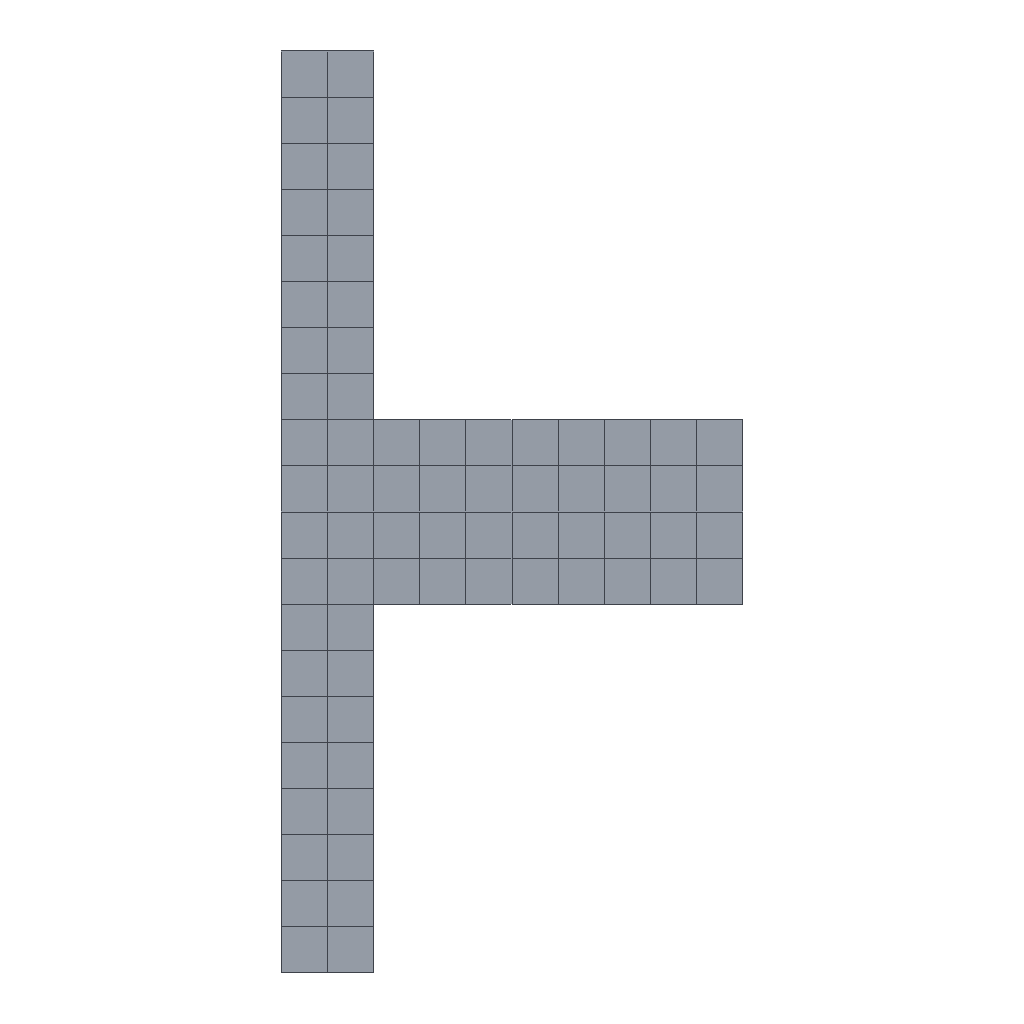Simulation study | abaqus
Set-up summary:
category,name,step,type,value,unit,region
solver,abaqus,,Abaqus/CAE 2024
units,SI m-kg-s (Pa),,inferred,E=2.10439e+11 density=
analysis,deadLoad,,static,nlgeom=True; time_period=1
analysis,heat1,,static,nlgeom=True; time_period=1
analysis,cool1,,static,nlgeom=True; time_period=1
analysis,heat2,,static,nlgeom=True; time_period=1
analysis,cool2,,static,nlgeom=True; time_period=1
analysis,heat3,,static,nlgeom=True; time_period=1
analysis,cool3,,static,nlgeom=True; time_period=1
analysis,heat4,,static,nlgeom=True; time_period=1
analysis,cool4,,static,nlgeom=True; time_period=1
mesh,nodes,,,114
mesh,elements,,,72
element_type,CAX4I,,,72
material,steel,,E,2.10439e+11
material,steel,,nu,0.3
material,steel,,yield,2e+08
material,steel,,cte,2e-05
material,steel,,behaviors,plastic; expansion; cyclic hardening
section,steel,,solid section,,,_PickedSet2
section,steel,,solid section,,,_PickedSet2
load,Load-1,deadLoad,pressure,-4.9735e+07,,press
load,Field-1,deadLoad,temperature,20,,all
load,Field-1,heat1,temperature,350,,all
load,Field-1,cool1,temperature,25,,all
load,Field-1,heat2,temperature,350,,all
load,Field-1,cool2,temperature,25,,all
load,Field-1,heat3,temperature,350,,all
load,Field-1,cool3,temperature,25,,all
load,Field-1,heat4,temperature,350,,all
load,Field-1,cool4,temperature,25,,all
bc,fixRB,deadLoad,fixed,[dofs=y],,fix
bc,fixTops,heat1,velocity,[dofs=y],,tops
contact,Int-1,initial,contact pair,interaction=fric; friction=0.1; behavior=hard,,topFlange / botFlange
constraint,equation,,,2
Abaqus input file, long lists of numbers shortened:
*Heading
** Job name: deck Model name: flange_comb
** Generated by: Abaqus/CAE 2024
*Preprint, echo=NO, model=NO, history=NO, contact=NO
**
** PARTS
**
*Part, name=botFlange
*End Part
**
*Part, name=topFlange
*End Part
**
**
** ASSEMBLY
**
*Assembly, name=Assembly
**
*Instance, name=botFlange-1, part=botFlange
*Node
      1, 0.09, -0.02
      2,  0.13, -0.02
** (55 more lines like these left out)
*Element, type=CAX4I
1,  1, 10, 42,  4
2, 10, 11, 43, 42
** (34 more lines like these left out)
*Nset, nset=_PickedSet2, internal, generate
  1,  57,   1
*Elset, elset=_PickedSet2, internal, generate
  1,  36,   1
** Section: Section-1
*Solid Section, elset=_PickedSet2, material=steel
1.,
*End Instance
**
*Instance, name=topFlange-1, part=topFlange
*Node
      1, 0.09,           0.
      2,  0.13,           0.
** (55 more lines like these left out)
*Element, type=CAX4I
1,  1, 10, 42,  4
2, 10, 11, 43, 42
** (34 more lines like these left out)
*Nset, nset=_PickedSet2, internal, generate
  1,  57,   1
*Elset, elset=_PickedSet2, internal, generate
  1,  36,   1
** Section: Section-1
*Solid Section, elset=_PickedSet2, material=steel
1.,
*End Instance
**
*Nset, nset=all, instance=botFlange-1, generate
  1,  57,   1
*Nset, nset=all, instance=topFlange-1, generate
  1,  57,   1
*Elset, elset=all, instance=botFlange-1, generate
  1,  36,   1
*Elset, elset=all, instance=topFlange-1, generate
  1,  36,   1
*Nset, nset=botBolt, instance=botFlange-1
 4,
*Nset, nset=fix, instance=topFlange-1
 6,
*Nset, nset=topBolt, instance=topFlange-1
 4,
*Nset, nset=tops, instance=botFlange-1
  7,  8, 31
*Nset, nset=tops, instance=topFlange-1
  7,  8, 27
*Elset, elset=tops, instance=botFlange-1
 23, 24
*Elset, elset=tops, instance=topFlange-1
 26, 36
*Elset, elset=_botFlange_S3, internal, instance=botFlange-1
  5,  6,  7,  8, 31, 32, 33, 34, 35, 36
*Surface, type=ELEMENT, name=botFlange
_botFlange_S3, S3
*Elset, elset=_press_S3, internal, instance=botFlange-1
 23, 24
*Elset, elset=_press_S2, internal, instance=topFlange-1
 26, 36
*Surface, type=ELEMENT, name=press
_press_S3, S3
_press_S2, S2
*Elset, elset=_topFlange_S1, internal, instance=topFlange-1, generate
 1,  4,  1
*Elset, elset=_topFlange_S2, internal, instance=topFlange-1, generate
 10,  16,   2
*Elset, elset=_topFlange_S4, internal, instance=topFlange-1
 17, 27
*Surface, type=ELEMENT, name=topFlange
_topFlange_S1, S1
_topFlange_S2, S2
_topFlange_S4, S4
** Constraint: tie bolt 1
*Equation
2
topBolt, 1, 1.
botBolt, 1, -1.
** Constraint: tie bolt 2
*Equation
2
topBolt, 2, 1.
botBolt, 2, -1.
*End Assembly
**
** MATERIALS
**
*Material, name=steel
*Elastic
 2.10439e+11, 0.3
*Expansion
 2e-05,
*Plastic, hardening=COMBINED, datatype=PARAMETERS, number backstresses=1
 2e+08, 2.55e+10,      81.
*Cyclic Hardening, parameters
 2e+08, 8e+08,  0.94
**
** INTERACTION PROPERTIES
**
*Surface Interaction, name=fric
1.,
*Friction, slip tolerance=0.005
 0.1,
*Surface Behavior, pressure-overclosure=HARD
**
** INTERACTIONS
**
** Interaction: Int-1
*Contact Pair, interaction=fric, small sliding
topFlange, botFlange
** ----------------------------------------------------------------
**
** STEP: deadLoad
**
*Step, name=deadLoad, nlgeom=YES
apply dead load of pipe weight
*Static
0.1, 1., 1e-05, 1.
**
** BOUNDARY CONDITIONS
**
** Name: fixRB Type: Displacement/Rotation
*Boundary
fix, 2, 2
**
** LOADS
**
** Name: Load-1   Type: Pressure
*Dsload
press, P, -4.9735e+07
**
** PREDEFINED FIELDS
**
** Name: Field-1   Type: Temperature
*Temperature
all, 20.
**
** OUTPUT REQUESTS
**
*Restart, write, frequency=0
**
** FIELD OUTPUT: F-Output-1
**
*Output, field, variable=PRESELECT
**
** HISTORY OUTPUT: H-Output-1
**
*Output, history, variable=PRESELECT
*End Step
** ----------------------------------------------------------------
**
** STEP: heat1
**
*Step, name=heat1, nlgeom=YES
1st heat up cycle
*Static
0.05, 1., 1e-05, 1.
**
** BOUNDARY CONDITIONS
**
** Name: fixRB Type: Displacement/Rotation
*Boundary, op=NEW
** Name: fixTops Type: Velocity/Angular velocity
*Boundary, op=NEW, type=VELOCITY
tops, 2, 2
**
** LOADS
**
** Name: Load-1   Type: Pressure
*Dsload, op=NEW
**
** PREDEFINED FIELDS
**
** Name: Field-1   Type: Temperature
*Temperature
all, 350.
**
** OUTPUT REQUESTS
**
*Restart, write, frequency=0
**
** FIELD OUTPUT: F-Output-1
**
*Output, field, variable=PRESELECT
**
** HISTORY OUTPUT: H-Output-1
**
*Output, history, variable=PRESELECT
*End Step
** ----------------------------------------------------------------
**
** STEP: cool1
**
*Step, name=cool1, nlgeom=YES
1st cooling cycle
*Static
0.05, 1., 1e-05, 1.
**
** PREDEFINED FIELDS
**
** Name: Field-1   Type: Temperature
*Temperature
all, 25.
**
** OUTPUT REQUESTS
**
*Restart, write, frequency=0
**
** FIELD OUTPUT: F-Output-1
**
*Output, field, variable=PRESELECT
**
** HISTORY OUTPUT: H-Output-1
**
*Output, history, variable=PRESELECT
*End Step
** ----------------------------------------------------------------
**
** STEP: heat2
**
*Step, name=heat2, nlgeom=YES
2nd heat up cycle
*Static
0.05, 1., 1e-05, 1.
**
** PREDEFINED FIELDS
**
** Name: Field-1   Type: Temperature
*Temperature
all, 350.
**
** OUTPUT REQUESTS
**
*Restart, write, frequency=0
**
** FIELD OUTPUT: F-Output-1
**
*Output, field, variable=PRESELECT
**
** HISTORY OUTPUT: H-Output-1
**
*Output, history, variable=PRESELECT
*End Step
** ----------------------------------------------------------------
**
** STEP: cool2
**
*Step, name=cool2, nlgeom=YES
2nd cooling cycle
*Static
0.05, 1., 1e-05, 1.
**
** PREDEFINED FIELDS
**
** Name: Field-1   Type: Temperature
*Temperature
all, 25.
**
** OUTPUT REQUESTS
**
*Restart, write, frequency=0
**
** FIELD OUTPUT: F-Output-1
**
*Output, field, variable=PRESELECT
**
** HISTORY OUTPUT: H-Output-1
**
*Output, history, variable=PRESELECT
*End Step
** ----------------------------------------------------------------
**
** STEP: heat3
**
*Step, name=heat3, nlgeom=YES
3rd heat up cycle
*Static
0.05, 1., 1e-05, 1.
**
** PREDEFINED FIELDS
**
** Name: Field-1   Type: Temperature
*Temperature
all, 350.
**
** OUTPUT REQUESTS
**
*Restart, write, frequency=0
**
** FIELD OUTPUT: F-Output-1
**
*Output, field, variable=PRESELECT
**
** HISTORY OUTPUT: H-Output-1
**
*Output, history, variable=PRESELECT
*End Step
** ----------------------------------------------------------------
**
** STEP: cool3
**
*Step, name=cool3, nlgeom=YES
3rd cooling cycle
*Static
0.05, 1., 1e-05, 1.
**
** PREDEFINED FIELDS
**
** Name: Field-1   Type: Temperature
*Temperature
all, 25.
**
** OUTPUT REQUESTS
**
*Restart, write, frequency=0
**
** FIELD OUTPUT: F-Output-1
**
*Output, field, variable=PRESELECT
**
** HISTORY OUTPUT: H-Output-1
**
*Output, history, variable=PRESELECT
*End Step
** ----------------------------------------------------------------
**
** STEP: heat4
**
*Step, name=heat4, nlgeom=YES
4th heat up cycle
*Static
0.05, 1., 1e-05, 1.
**
** PREDEFINED FIELDS
**
** Name: Field-1   Type: Temperature
*Temperature
all, 350.
**
** OUTPUT REQUESTS
**
*Restart, write, frequency=0
**
** FIELD OUTPUT: F-Output-1
**
*Output, field, variable=PRESELECT
**
** HISTORY OUTPUT: H-Output-1
**
*Output, history, variable=PRESELECT
*End Step
** ----------------------------------------------------------------
**
** STEP: cool4
**
*Step, name=cool4, nlgeom=YES
4th cooling cycle
*Static
0.05, 1., 1e-05, 1.
**
** PREDEFINED FIELDS
**
** Name: Field-1   Type: Temperature
*Temperature
all, 25.
**
** OUTPUT REQUESTS
**
*Restart, write, frequency=0
**
** FIELD OUTPUT: F-Output-1
**
*Output, field, variable=PRESELECT
**
** HISTORY OUTPUT: H-Output-1
**
*Output, history, variable=PRESELECT
*End Step
Results summary, first 51 of 100 lines:
result,odb.job_status,,,JOB_STATUS_COMPLETED_SUCCESSFULLY,"consistent, unstated (Abaqus has no unit system)"
result,steps[0].procedure,deadLoad,,*STATIC,"consistent, unstated (Abaqus has no unit system)"
result,steps[0].time_period,deadLoad,,1,"consistent, unstated (Abaqus has no unit system)"
result,steps[0].n_frames,deadLoad,,7,"consistent, unstated (Abaqus has no unit system)"
result,steps[0].last_frame.id,deadLoad,,6,"consistent, unstated (Abaqus has no unit system)"
result,steps[0].last_frame.value,deadLoad,,1,"consistent, unstated (Abaqus has no unit system)"
result,steps[0].last_frame.description,deadLoad,,Increment      6: Step Time =    1.000,"consistent, unstated (Abaqus has no unit system)"
result,steps[0].completed,deadLoad,,True,"consistent, unstated (Abaqus has no unit system)"
result,steps[0].max_U_magnitude,deadLoad,,0.0002134,"consistent, unstated (Abaqus has no unit system)"
result,steps[0].max_S_mises,deadLoad,,1.48728e+08,"consistent, unstated (Abaqus has no unit system)"
result,steps[0].RF_sum[1],deadLoad,,0,"consistent, unstated (Abaqus has no unit system)"
result,steps[0].RF_sum[2],deadLoad,,-0.02349,"consistent, unstated (Abaqus has no unit system)"
result,steps[1].procedure,heat1,,*STATIC,"consistent, unstated (Abaqus has no unit system)"
result,steps[1].time_period,heat1,,1,"consistent, unstated (Abaqus has no unit system)"
result,steps[1].n_frames,heat1,,8,"consistent, unstated (Abaqus has no unit system)"
result,steps[1].last_frame.id,heat1,,7,"consistent, unstated (Abaqus has no unit system)"
result,steps[1].last_frame.value,heat1,,1,"consistent, unstated (Abaqus has no unit system)"
result,steps[1].last_frame.description,heat1,,Increment      7: Step Time =    1.000,"consistent, unstated (Abaqus has no unit system)"
result,steps[1].completed,heat1,,True,"consistent, unstated (Abaqus has no unit system)"
result,steps[1].max_U_magnitude,heat1,,0.001012,"consistent, unstated (Abaqus has no unit system)"
result,steps[1].max_S_mises,heat1,,3.39584e+08,"consistent, unstated (Abaqus has no unit system)"
result,steps[1].RF_sum[1],heat1,,0,"consistent, unstated (Abaqus has no unit system)"
result,steps[1].RF_sum[2],heat1,,0,"consistent, unstated (Abaqus has no unit system)"
result,steps[2].procedure,cool1,,*STATIC,"consistent, unstated (Abaqus has no unit system)"
result,steps[2].time_period,cool1,,1,"consistent, unstated (Abaqus has no unit system)"
result,steps[2].n_frames,cool1,,8,"consistent, unstated (Abaqus has no unit system)"
result,steps[2].last_frame.id,cool1,,7,"consistent, unstated (Abaqus has no unit system)"
result,steps[2].last_frame.value,cool1,,1,"consistent, unstated (Abaqus has no unit system)"
result,steps[2].last_frame.description,cool1,,Increment      7: Step Time =    1.000,"consistent, unstated (Abaqus has no unit system)"
result,steps[2].completed,cool1,,True,"consistent, unstated (Abaqus has no unit system)"
result,steps[2].max_U_magnitude,cool1,,0.0005642,"consistent, unstated (Abaqus has no unit system)"
result,steps[2].max_S_mises,cool1,,2.52138e+08,"consistent, unstated (Abaqus has no unit system)"
result,steps[2].RF_sum[1],cool1,,0,"consistent, unstated (Abaqus has no unit system)"
result,steps[2].RF_sum[2],cool1,,-0.03125,"consistent, unstated (Abaqus has no unit system)"
result,steps[3].procedure,heat2,,*STATIC,"consistent, unstated (Abaqus has no unit system)"
result,steps[3].time_period,heat2,,1,"consistent, unstated (Abaqus has no unit system)"
result,steps[3].n_frames,heat2,,10,"consistent, unstated (Abaqus has no unit system)"
result,steps[3].last_frame.id,heat2,,9,"consistent, unstated (Abaqus has no unit system)"
result,steps[3].last_frame.value,heat2,,1,"consistent, unstated (Abaqus has no unit system)"
result,steps[3].last_frame.description,heat2,,Increment      9: Step Time =    1.000,"consistent, unstated (Abaqus has no unit system)"
result,steps[3].completed,heat2,,True,"consistent, unstated (Abaqus has no unit system)"
result,steps[3].max_U_magnitude,heat2,,0.001014,"consistent, unstated (Abaqus has no unit system)"
result,steps[3].max_S_mises,heat2,,3.25198e+08,"consistent, unstated (Abaqus has no unit system)"
result,steps[3].RF_sum[1],heat2,,0,"consistent, unstated (Abaqus has no unit system)"
result,steps[3].RF_sum[2],heat2,,0.0625,"consistent, unstated (Abaqus has no unit system)"
result,steps[4].procedure,cool2,,*STATIC,"consistent, unstated (Abaqus has no unit system)"
result,steps[4].time_period,cool2,,1,"consistent, unstated (Abaqus has no unit system)"
result,steps[4].n_frames,cool2,,11,"consistent, unstated (Abaqus has no unit system)"
result,steps[4].last_frame.id,cool2,,10,"consistent, unstated (Abaqus has no unit system)"
result,steps[4].last_frame.value,cool2,,1,"consistent, unstated (Abaqus has no unit system)"
result,steps[4].last_frame.description,cool2,,Increment     10: Step Time =    1.000,"consistent, unstated (Abaqus has no unit system)"